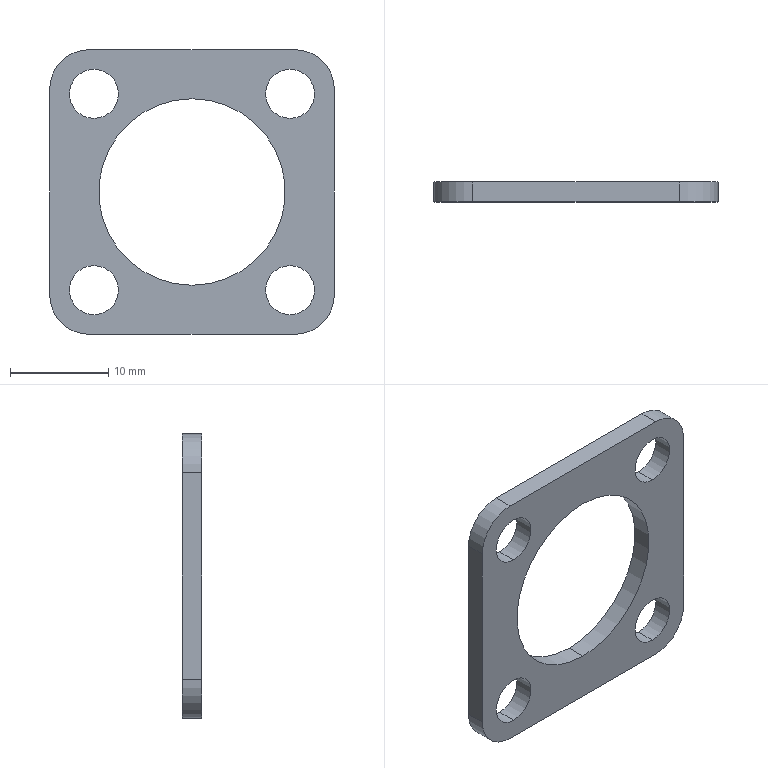Part | NX | features BREP 1 | 1 solid | 20 faces | box 29 x 2 x 29 mm | volume 930.394 mm3 | cylinder 14 | plane 6 | commonest cylinder face diameters 5 x8 8 x4 19 x2
STEP:
#1=CARTESIAN_POINT('',(10.,2.,7.5));
#2=VERTEX_POINT('',#1);
#3=CARTESIAN_POINT('',(10.,2.,12.5));
#4=VERTEX_POINT('',#3);
#5=CARTESIAN_POINT('',(10.,2.,10.));
#6=DIRECTION('',(0.,1.,0.));
#7=DIRECTION('',(1.,0.,0.));
#8=AXIS2_PLACEMENT_3D('',#5,#6,#7);
#9=CIRCLE('',#8,2.5);
#10=EDGE_CURVE('',#2,#4,#9,.T.);
#11=ORIENTED_EDGE('',*,*,#10,.T.);
#12=CARTESIAN_POINT('',(10.,0.,12.5));
#13=VERTEX_POINT('',#12);
#14=CARTESIAN_POINT('',(10.,2.,12.5));
#15=DIRECTION('',(0.,1.,0.));
#16=VECTOR('',#15,1000.);
#17=LINE('',#14,#16);
#18=EDGE_CURVE('',#13,#4,#17,.T.);
#19=ORIENTED_EDGE('',*,*,#18,.F.);
#20=CARTESIAN_POINT('',(10.,0.,7.5));
#21=VERTEX_POINT('',#20);
#22=CARTESIAN_POINT('',(10.,0.,10.));
#23=DIRECTION('',(0.,1.,0.));
#24=DIRECTION('',(1.,0.,0.));
#25=AXIS2_PLACEMENT_3D('',#22,#23,#24);
#26=CIRCLE('',#25,2.5);
#27=EDGE_CURVE('',#21,#13,#26,.T.);
#28=ORIENTED_EDGE('',*,*,#27,.F.);
#29=CARTESIAN_POINT('',(10.,2.,7.5));
#30=DIRECTION('',(0.,1.,0.));
#31=VECTOR('',#30,1000.);
#32=LINE('',#29,#31);
#33=EDGE_CURVE('',#21,#2,#32,.T.);
#34=ORIENTED_EDGE('',*,*,#33,.T.);
#35=EDGE_LOOP('',(#11,#19,#28,#34));
#36=FACE_BOUND('',#35,.T.);
#37=CARTESIAN_POINT('',(10.,2.,10.));
#38=DIRECTION('',(0.,-1.,0.));
#39=DIRECTION('',(0.,0.,-1.));
#40=AXIS2_PLACEMENT_3D('',#37,#38,#39);
#41=CYLINDRICAL_SURFACE('',#40,2.5);
#42=ADVANCED_FACE('',(#36),#41,.F.);
#43=CARTESIAN_POINT('',(10.5,2.,14.5));
#44=VERTEX_POINT('',#43);
#45=CARTESIAN_POINT('',(14.5,2.,10.5));
#46=VERTEX_POINT('',#45);
#47=CARTESIAN_POINT('',(10.5,2.,10.5));
#48=DIRECTION('',(0.,1.,0.));
#49=DIRECTION('',(1.,0.,0.));
#50=AXIS2_PLACEMENT_3D('',#47,#48,#49);
#51=CIRCLE('',#50,4.);
#52=EDGE_CURVE('',#44,#46,#51,.T.);
#53=ORIENTED_EDGE('',*,*,#52,.T.);
#54=CARTESIAN_POINT('',(14.5,2.,-10.5));
#55=VERTEX_POINT('',#54);
#56=CARTESIAN_POINT('',(14.5,2.,0.));
#57=DIRECTION('',(0.,0.,-1.));
#58=VECTOR('',#57,1000.);
#59=LINE('',#56,#58);
#60=EDGE_CURVE('',#46,#55,#59,.T.);
#61=ORIENTED_EDGE('',*,*,#60,.T.);
#62=CARTESIAN_POINT('',(10.5,2.,-14.5));
#63=VERTEX_POINT('',#62);
#64=CARTESIAN_POINT('',(10.5,2.,-10.5));
#65=DIRECTION('',(0.,1.,0.));
#66=DIRECTION('',(1.,0.,0.));
#67=AXIS2_PLACEMENT_3D('',#64,#65,#66);
#68=CIRCLE('',#67,4.);
#69=EDGE_CURVE('',#55,#63,#68,.T.);
#70=ORIENTED_EDGE('',*,*,#69,.T.);
#71=CARTESIAN_POINT('',(-10.5,2.,-14.5));
#72=VERTEX_POINT('',#71);
#73=CARTESIAN_POINT('',(0.,2.,-14.5));
#74=DIRECTION('',(-1.,0.,0.));
#75=VECTOR('',#74,1000.);
#76=LINE('',#73,#75);
#77=EDGE_CURVE('',#63,#72,#76,.T.);
#78=ORIENTED_EDGE('',*,*,#77,.T.);
#79=CARTESIAN_POINT('',(-14.5,2.,-10.5));
#80=VERTEX_POINT('',#79);
#81=CARTESIAN_POINT('',(-10.5,2.,-10.5));
#82=DIRECTION('',(0.,1.,0.));
#83=DIRECTION('',(1.,0.,0.));
#84=AXIS2_PLACEMENT_3D('',#81,#82,#83);
#85=CIRCLE('',#84,4.);
#86=EDGE_CURVE('',#72,#80,#85,.T.);
#87=ORIENTED_EDGE('',*,*,#86,.T.);
#88=CARTESIAN_POINT('',(-14.5,2.,10.5));
#89=VERTEX_POINT('',#88);
#90=CARTESIAN_POINT('',(-14.5,2.,0.));
#91=DIRECTION('',(0.,0.,1.));
#92=VECTOR('',#91,1000.);
#93=LINE('',#90,#92);
#94=EDGE_CURVE('',#80,#89,#93,.T.);
#95=ORIENTED_EDGE('',*,*,#94,.T.);
#96=CARTESIAN_POINT('',(-10.5,2.,14.5));
#97=VERTEX_POINT('',#96);
#98=CARTESIAN_POINT('',(-10.5,2.,10.5));
#99=DIRECTION('',(0.,1.,0.));
#100=DIRECTION('',(1.,0.,0.));
#101=AXIS2_PLACEMENT_3D('',#98,#99,#100);
#102=CIRCLE('',#101,4.);
#103=EDGE_CURVE('',#89,#97,#102,.T.);
#104=ORIENTED_EDGE('',*,*,#103,.T.);
#105=CARTESIAN_POINT('',(0.,2.,14.5));
#106=DIRECTION('',(1.,0.,0.));
#107=VECTOR('',#106,1000.);
#108=LINE('',#105,#107);
#109=EDGE_CURVE('',#97,#44,#108,.T.);
#110=ORIENTED_EDGE('',*,*,#109,.T.);
#111=EDGE_LOOP('',(#53,#61,#70,#78,#87,#95,#104,#110));
#112=FACE_BOUND('',#111,.T.);
#113=CARTESIAN_POINT('',(10.,2.,-12.5));
#114=VERTEX_POINT('',#113);
#115=CARTESIAN_POINT('',(10.,2.,-7.5));
#116=VERTEX_POINT('',#115);
#117=CARTESIAN_POINT('',(10.,2.,-10.));
#118=DIRECTION('',(0.,1.,0.));
#119=DIRECTION('',(1.,0.,0.));
#120=AXIS2_PLACEMENT_3D('',#117,#118,#119);
#121=CIRCLE('',#120,2.5);
#122=EDGE_CURVE('',#114,#116,#121,.T.);
#123=ORIENTED_EDGE('',*,*,#122,.F.);
#124=CARTESIAN_POINT('',(10.,2.,-10.));
#125=DIRECTION('',(0.,1.,0.));
#126=DIRECTION('',(1.,0.,0.));
#127=AXIS2_PLACEMENT_3D('',#124,#125,#126);
#128=CIRCLE('',#127,2.5);
#129=EDGE_CURVE('',#116,#114,#128,.T.);
#130=ORIENTED_EDGE('',*,*,#129,.F.);
#131=EDGE_LOOP('',(#123,#130));
#132=FACE_BOUND('',#131,.T.);
#133=CARTESIAN_POINT('',(-10.,2.,-12.5));
#134=VERTEX_POINT('',#133);
#135=CARTESIAN_POINT('',(-10.,2.,-7.5));
#136=VERTEX_POINT('',#135);
#137=CARTESIAN_POINT('',(-10.,2.,-10.));
#138=DIRECTION('',(0.,1.,0.));
#139=DIRECTION('',(1.,0.,0.));
#140=AXIS2_PLACEMENT_3D('',#137,#138,#139);
#141=CIRCLE('',#140,2.5);
#142=EDGE_CURVE('',#134,#136,#141,.T.);
#143=ORIENTED_EDGE('',*,*,#142,.F.);
#144=CARTESIAN_POINT('',(-10.,2.,-10.));
#145=DIRECTION('',(0.,1.,0.));
#146=DIRECTION('',(1.,0.,0.));
#147=AXIS2_PLACEMENT_3D('',#144,#145,#146);
#148=CIRCLE('',#147,2.5);
#149=EDGE_CURVE('',#136,#134,#148,.T.);
#150=ORIENTED_EDGE('',*,*,#149,.F.);
#151=EDGE_LOOP('',(#143,#150));
#152=FACE_BOUND('',#151,.T.);
#153=CARTESIAN_POINT('',(0.,2.,-9.5));
#154=VERTEX_POINT('',#153);
#155=CARTESIAN_POINT('',(0.,2.,9.5));
#156=VERTEX_POINT('',#155);
#157=CARTESIAN_POINT('',(0.,2.,0.));
#158=DIRECTION('',(0.,1.,0.));
#159=DIRECTION('',(1.,0.,0.));
#160=AXIS2_PLACEMENT_3D('',#157,#158,#159);
#161=CIRCLE('',#160,9.5);
#162=EDGE_CURVE('',#154,#156,#161,.T.);
#163=ORIENTED_EDGE('',*,*,#162,.F.);
#164=CARTESIAN_POINT('',(0.,2.,0.));
#165=DIRECTION('',(0.,1.,0.));
#166=DIRECTION('',(1.,0.,0.));
#167=AXIS2_PLACEMENT_3D('',#164,#165,#166);
#168=CIRCLE('',#167,9.5);
#169=EDGE_CURVE('',#156,#154,#168,.T.);
#170=ORIENTED_EDGE('',*,*,#169,.F.);
#171=EDGE_LOOP('',(#163,#170));
#172=FACE_BOUND('',#171,.T.);
#173=CARTESIAN_POINT('',(-10.,2.,7.5));
#174=VERTEX_POINT('',#173);
#175=CARTESIAN_POINT('',(-10.,2.,12.5));
#176=VERTEX_POINT('',#175);
#177=CARTESIAN_POINT('',(-10.,2.,10.));
#178=DIRECTION('',(0.,1.,0.));
#179=DIRECTION('',(1.,0.,0.));
#180=AXIS2_PLACEMENT_3D('',#177,#178,#179);
#181=CIRCLE('',#180,2.5);
#182=EDGE_CURVE('',#174,#176,#181,.T.);
#183=ORIENTED_EDGE('',*,*,#182,.F.);
#184=CARTESIAN_POINT('',(-10.,2.,10.));
#185=DIRECTION('',(0.,1.,0.));
#186=DIRECTION('',(1.,0.,0.));
#187=AXIS2_PLACEMENT_3D('',#184,#185,#186);
#188=CIRCLE('',#187,2.5);
#189=EDGE_CURVE('',#176,#174,#188,.T.);
#190=ORIENTED_EDGE('',*,*,#189,.F.);
#191=EDGE_LOOP('',(#183,#190));
#192=FACE_BOUND('',#191,.T.);
#193=ORIENTED_EDGE('',*,*,#10,.F.);
#194=CARTESIAN_POINT('',(10.,2.,10.));
#195=DIRECTION('',(0.,1.,0.));
#196=DIRECTION('',(1.,0.,0.));
#197=AXIS2_PLACEMENT_3D('',#194,#195,#196);
#198=CIRCLE('',#197,2.5);
#199=EDGE_CURVE('',#4,#2,#198,.T.);
#200=ORIENTED_EDGE('',*,*,#199,.F.);
#201=EDGE_LOOP('',(#193,#200));
#202=FACE_BOUND('',#201,.T.);
#203=CARTESIAN_POINT('',(10.5,2.,10.5));
#204=DIRECTION('',(0.,1.,0.));
#205=DIRECTION('',(0.,0.,-1.));
#206=AXIS2_PLACEMENT_3D('',#203,#204,#205);
#207=PLANE('',#206);
#208=ADVANCED_FACE('',(#112,#132,#152,#172,#192,#202),#207,.T.);
#209=ORIENTED_EDGE('',*,*,#18,.T.);
#210=ORIENTED_EDGE('',*,*,#199,.T.);
#211=ORIENTED_EDGE('',*,*,#33,.F.);
#212=CARTESIAN_POINT('',(10.,0.,10.));
#213=DIRECTION('',(0.,1.,0.));
#214=DIRECTION('',(1.,0.,0.));
#215=AXIS2_PLACEMENT_3D('',#212,#213,#214);
#216=CIRCLE('',#215,2.5);
#217=EDGE_CURVE('',#13,#21,#216,.T.);
#218=ORIENTED_EDGE('',*,*,#217,.F.);
#219=EDGE_LOOP('',(#209,#210,#211,#218));
#220=FACE_BOUND('',#219,.T.);
#221=CARTESIAN_POINT('',(10.,2.,10.));
#222=DIRECTION('',(0.,-1.,0.));
#223=DIRECTION('',(0.,0.,1.));
#224=AXIS2_PLACEMENT_3D('',#221,#222,#223);
#225=CYLINDRICAL_SURFACE('',#224,2.5);
#226=ADVANCED_FACE('',(#220),#225,.F.);
#227=CARTESIAN_POINT('',(10.5,0.,14.5));
#228=VERTEX_POINT('',#227);
#229=CARTESIAN_POINT('',(14.5,0.,10.5));
#230=VERTEX_POINT('',#229);
#231=CARTESIAN_POINT('',(10.5,0.,10.5));
#232=DIRECTION('',(0.,1.,0.));
#233=DIRECTION('',(1.,0.,0.));
#234=AXIS2_PLACEMENT_3D('',#231,#232,#233);
#235=CIRCLE('',#234,4.);
#236=EDGE_CURVE('',#228,#230,#235,.T.);
#237=ORIENTED_EDGE('',*,*,#236,.F.);
#238=CARTESIAN_POINT('',(-10.5,0.,14.5));
#239=VERTEX_POINT('',#238);
#240=CARTESIAN_POINT('',(0.,0.,14.5));
#241=DIRECTION('',(1.,0.,0.));
#242=VECTOR('',#241,1000.);
#243=LINE('',#240,#242);
#244=EDGE_CURVE('',#239,#228,#243,.T.);
#245=ORIENTED_EDGE('',*,*,#244,.F.);
#246=CARTESIAN_POINT('',(-14.5,0.,10.5));
#247=VERTEX_POINT('',#246);
#248=CARTESIAN_POINT('',(-10.5,0.,10.5));
#249=DIRECTION('',(0.,1.,0.));
#250=DIRECTION('',(1.,0.,0.));
#251=AXIS2_PLACEMENT_3D('',#248,#249,#250);
#252=CIRCLE('',#251,4.);
#253=EDGE_CURVE('',#247,#239,#252,.T.);
#254=ORIENTED_EDGE('',*,*,#253,.F.);
#255=CARTESIAN_POINT('',(-14.5,0.,-10.5));
#256=VERTEX_POINT('',#255);
#257=CARTESIAN_POINT('',(-14.5,0.,0.));
#258=DIRECTION('',(0.,0.,1.));
#259=VECTOR('',#258,1000.);
#260=LINE('',#257,#259);
#261=EDGE_CURVE('',#256,#247,#260,.T.);
#262=ORIENTED_EDGE('',*,*,#261,.F.);
#263=CARTESIAN_POINT('',(-10.5,0.,-14.5));
#264=VERTEX_POINT('',#263);
#265=CARTESIAN_POINT('',(-10.5,0.,-10.5));
#266=DIRECTION('',(0.,1.,0.));
#267=DIRECTION('',(1.,0.,0.));
#268=AXIS2_PLACEMENT_3D('',#265,#266,#267);
#269=CIRCLE('',#268,4.);
#270=EDGE_CURVE('',#264,#256,#269,.T.);
#271=ORIENTED_EDGE('',*,*,#270,.F.);
#272=CARTESIAN_POINT('',(10.5,0.,-14.5));
#273=VERTEX_POINT('',#272);
#274=CARTESIAN_POINT('',(0.,0.,-14.5));
#275=DIRECTION('',(-1.,0.,0.));
#276=VECTOR('',#275,1000.);
#277=LINE('',#274,#276);
#278=EDGE_CURVE('',#273,#264,#277,.T.);
#279=ORIENTED_EDGE('',*,*,#278,.F.);
#280=CARTESIAN_POINT('',(14.5,0.,-10.5));
#281=VERTEX_POINT('',#280);
#282=CARTESIAN_POINT('',(10.5,0.,-10.5));
#283=DIRECTION('',(0.,1.,0.));
#284=DIRECTION('',(1.,0.,0.));
#285=AXIS2_PLACEMENT_3D('',#282,#283,#284);
#286=CIRCLE('',#285,4.);
#287=EDGE_CURVE('',#281,#273,#286,.T.);
#288=ORIENTED_EDGE('',*,*,#287,.F.);
#289=CARTESIAN_POINT('',(14.5,0.,0.));
#290=DIRECTION('',(0.,0.,-1.));
#291=VECTOR('',#290,1000.);
#292=LINE('',#289,#291);
#293=EDGE_CURVE('',#230,#281,#292,.T.);
#294=ORIENTED_EDGE('',*,*,#293,.F.);
#295=EDGE_LOOP('',(#237,#245,#254,#262,#271,#279,#288,#294));
#296=FACE_BOUND('',#295,.T.);
#297=CARTESIAN_POINT('',(0.,0.,-9.5));
#298=VERTEX_POINT('',#297);
#299=CARTESIAN_POINT('',(0.,0.,9.5));
#300=VERTEX_POINT('',#299);
#301=CARTESIAN_POINT('',(0.,0.,0.));
#302=DIRECTION('',(0.,1.,0.));
#303=DIRECTION('',(1.,0.,0.));
#304=AXIS2_PLACEMENT_3D('',#301,#302,#303);
#305=CIRCLE('',#304,9.5);
#306=EDGE_CURVE('',#298,#300,#305,.T.);
#307=ORIENTED_EDGE('',*,*,#306,.T.);
#308=CARTESIAN_POINT('',(0.,0.,0.));
#309=DIRECTION('',(0.,1.,0.));
#310=DIRECTION('',(1.,0.,0.));
#311=AXIS2_PLACEMENT_3D('',#308,#309,#310);
#312=CIRCLE('',#311,9.5);
#313=EDGE_CURVE('',#300,#298,#312,.T.);
#314=ORIENTED_EDGE('',*,*,#313,.T.);
#315=EDGE_LOOP('',(#307,#314));
#316=FACE_BOUND('',#315,.T.);
#317=CARTESIAN_POINT('',(-10.,0.,-12.5));
#318=VERTEX_POINT('',#317);
#319=CARTESIAN_POINT('',(-10.,0.,-7.5));
#320=VERTEX_POINT('',#319);
#321=CARTESIAN_POINT('',(-10.,0.,-10.));
#322=DIRECTION('',(0.,1.,0.));
#323=DIRECTION('',(1.,0.,0.));
#324=AXIS2_PLACEMENT_3D('',#321,#322,#323);
#325=CIRCLE('',#324,2.5);
#326=EDGE_CURVE('',#318,#320,#325,.T.);
#327=ORIENTED_EDGE('',*,*,#326,.T.);
#328=CARTESIAN_POINT('',(-10.,0.,-10.));
#329=DIRECTION('',(0.,1.,0.));
#330=DIRECTION('',(1.,0.,0.));
#331=AXIS2_PLACEMENT_3D('',#328,#329,#330);
#332=CIRCLE('',#331,2.5);
#333=EDGE_CURVE('',#320,#318,#332,.T.);
#334=ORIENTED_EDGE('',*,*,#333,.T.);
#335=EDGE_LOOP('',(#327,#334));
#336=FACE_BOUND('',#335,.T.);
#337=CARTESIAN_POINT('',(-10.,0.,7.5));
#338=VERTEX_POINT('',#337);
#339=CARTESIAN_POINT('',(-10.,0.,12.5));
#340=VERTEX_POINT('',#339);
#341=CARTESIAN_POINT('',(-10.,0.,10.));
#342=DIRECTION('',(0.,1.,0.));
#343=DIRECTION('',(1.,0.,0.));
#344=AXIS2_PLACEMENT_3D('',#341,#342,#343);
#345=CIRCLE('',#344,2.5);
#346=EDGE_CURVE('',#338,#340,#345,.T.);
#347=ORIENTED_EDGE('',*,*,#346,.T.);
#348=CARTESIAN_POINT('',(-10.,0.,10.));
#349=DIRECTION('',(0.,1.,0.));
#350=DIRECTION('',(1.,0.,0.));
#351=AXIS2_PLACEMENT_3D('',#348,#349,#350);
#352=CIRCLE('',#351,2.5);
#353=EDGE_CURVE('',#340,#338,#352,.T.);
#354=ORIENTED_EDGE('',*,*,#353,.T.);
#355=EDGE_LOOP('',(#347,#354));
#356=FACE_BOUND('',#355,.T.);
#357=CARTESIAN_POINT('',(10.,0.,-12.5));
#358=VERTEX_POINT('',#357);
#359=CARTESIAN_POINT('',(10.,0.,-7.5));
#360=VERTEX_POINT('',#359);
#361=CARTESIAN_POINT('',(10.,0.,-10.));
#362=DIRECTION('',(0.,1.,0.));
#363=DIRECTION('',(1.,0.,0.));
#364=AXIS2_PLACEMENT_3D('',#361,#362,#363);
#365=CIRCLE('',#364,2.5);
#366=EDGE_CURVE('',#358,#360,#365,.T.);
#367=ORIENTED_EDGE('',*,*,#366,.T.);
#368=CARTESIAN_POINT('',(10.,0.,-10.));
#369=DIRECTION('',(0.,1.,0.));
#370=DIRECTION('',(1.,0.,0.));
#371=AXIS2_PLACEMENT_3D('',#368,#369,#370);
#372=CIRCLE('',#371,2.5);
#373=EDGE_CURVE('',#360,#358,#372,.T.);
#374=ORIENTED_EDGE('',*,*,#373,.T.);
#375=EDGE_LOOP('',(#367,#374));
#376=FACE_BOUND('',#375,.T.);
#377=ORIENTED_EDGE('',*,*,#27,.T.);
#378=ORIENTED_EDGE('',*,*,#217,.T.);
#379=EDGE_LOOP('',(#377,#378));
#380=FACE_BOUND('',#379,.T.);
#381=CARTESIAN_POINT('',(10.5,0.,10.5));
#382=DIRECTION('',(0.,1.,0.));
#383=DIRECTION('',(0.,0.,-1.));
#384=AXIS2_PLACEMENT_3D('',#381,#382,#383);
#385=PLANE('',#384);
#386=ADVANCED_FACE('',(#296,#316,#336,#356,#376,#380),#385,.F.);
#387=ORIENTED_EDGE('',*,*,#236,.T.);
#388=CARTESIAN_POINT('',(14.5,2.,10.5));
#389=DIRECTION('',(0.,-1.,0.));
#390=VECTOR('',#389,1000.);
#391=LINE('',#388,#390);
#392=EDGE_CURVE('',#46,#230,#391,.T.);
#393=ORIENTED_EDGE('',*,*,#392,.F.);
#394=ORIENTED_EDGE('',*,*,#52,.F.);
#395=CARTESIAN_POINT('',(10.5,2.,14.5));
#396=DIRECTION('',(0.,-1.,0.));
#397=VECTOR('',#396,1000.);
#398=LINE('',#395,#397);
#399=EDGE_CURVE('',#44,#228,#398,.T.);
#400=ORIENTED_EDGE('',*,*,#399,.T.);
#401=EDGE_LOOP('',(#387,#393,#394,#400));
#402=FACE_BOUND('',#401,.T.);
#403=CARTESIAN_POINT('',(10.5,2.,10.5));
#404=DIRECTION('',(0.,-1.,0.));
#405=DIRECTION('',(0.,0.,1.));
#406=AXIS2_PLACEMENT_3D('',#403,#404,#405);
#407=CYLINDRICAL_SURFACE('',#406,4.);
#408=ADVANCED_FACE('',(#402),#407,.T.);
#409=ORIENTED_EDGE('',*,*,#293,.T.);
#410=CARTESIAN_POINT('',(14.5,1.,-10.5));
#411=DIRECTION('',(0.,-1.,0.));
#412=VECTOR('',#411,1000.);
#413=LINE('',#410,#412);
#414=EDGE_CURVE('',#55,#281,#413,.T.);
#415=ORIENTED_EDGE('',*,*,#414,.F.);
#416=ORIENTED_EDGE('',*,*,#60,.F.);
#417=ORIENTED_EDGE('',*,*,#392,.T.);
#418=EDGE_LOOP('',(#409,#415,#416,#417));
#419=FACE_BOUND('',#418,.T.);
#420=CARTESIAN_POINT('',(14.5,2.,10.5));
#421=DIRECTION('',(-1.,0.,0.));
#422=DIRECTION('',(0.,0.,-1.));
#423=AXIS2_PLACEMENT_3D('',#420,#421,#422);
#424=PLANE('',#423);
#425=ADVANCED_FACE('',(#419),#424,.F.);
#426=ORIENTED_EDGE('',*,*,#287,.T.);
#427=CARTESIAN_POINT('',(10.5,2.,-14.5));
#428=DIRECTION('',(0.,-1.,0.));
#429=VECTOR('',#428,1000.);
#430=LINE('',#427,#429);
#431=EDGE_CURVE('',#63,#273,#430,.T.);
#432=ORIENTED_EDGE('',*,*,#431,.F.);
#433=ORIENTED_EDGE('',*,*,#69,.F.);
#434=ORIENTED_EDGE('',*,*,#414,.T.);
#435=EDGE_LOOP('',(#426,#432,#433,#434));
#436=FACE_BOUND('',#435,.T.);
#437=CARTESIAN_POINT('',(10.5,2.,-10.5));
#438=DIRECTION('',(0.,-1.,0.));
#439=DIRECTION('',(0.,0.,1.));
#440=AXIS2_PLACEMENT_3D('',#437,#438,#439);
#441=CYLINDRICAL_SURFACE('',#440,4.);
#442=ADVANCED_FACE('',(#436),#441,.T.);
#443=ORIENTED_EDGE('',*,*,#278,.T.);
#444=CARTESIAN_POINT('',(-10.5,1.,-14.5));
#445=DIRECTION('',(0.,-1.,0.));
#446=VECTOR('',#445,1000.);
#447=LINE('',#444,#446);
#448=EDGE_CURVE('',#72,#264,#447,.T.);
#449=ORIENTED_EDGE('',*,*,#448,.F.);
#450=ORIENTED_EDGE('',*,*,#77,.F.);
#451=ORIENTED_EDGE('',*,*,#431,.T.);
#452=EDGE_LOOP('',(#443,#449,#450,#451));
#453=FACE_BOUND('',#452,.T.);
#454=CARTESIAN_POINT('',(-10.5,2.,-14.5));
#455=DIRECTION('',(0.,0.,1.));
#456=DIRECTION('',(-1.,0.,0.));
#457=AXIS2_PLACEMENT_3D('',#454,#455,#456);
#458=PLANE('',#457);
#459=ADVANCED_FACE('',(#453),#458,.F.);
#460=ORIENTED_EDGE('',*,*,#270,.T.);
#461=CARTESIAN_POINT('',(-14.5,2.,-10.5));
#462=DIRECTION('',(0.,-1.,0.));
#463=VECTOR('',#462,1000.);
#464=LINE('',#461,#463);
#465=EDGE_CURVE('',#80,#256,#464,.T.);
#466=ORIENTED_EDGE('',*,*,#465,.F.);
#467=ORIENTED_EDGE('',*,*,#86,.F.);
#468=ORIENTED_EDGE('',*,*,#448,.T.);
#469=EDGE_LOOP('',(#460,#466,#467,#468));
#470=FACE_BOUND('',#469,.T.);
#471=CARTESIAN_POINT('',(-10.5,2.,-10.5));
#472=DIRECTION('',(0.,-1.,0.));
#473=DIRECTION('',(0.,0.,-1.));
#474=AXIS2_PLACEMENT_3D('',#471,#472,#473);
#475=CYLINDRICAL_SURFACE('',#474,4.);
#476=ADVANCED_FACE('',(#470),#475,.T.);
#477=ORIENTED_EDGE('',*,*,#261,.T.);
#478=CARTESIAN_POINT('',(-14.5,1.,10.5));
#479=DIRECTION('',(0.,-1.,0.));
#480=VECTOR('',#479,1000.);
#481=LINE('',#478,#480);
#482=EDGE_CURVE('',#89,#247,#481,.T.);
#483=ORIENTED_EDGE('',*,*,#482,.F.);
#484=ORIENTED_EDGE('',*,*,#94,.F.);
#485=ORIENTED_EDGE('',*,*,#465,.T.);
#486=EDGE_LOOP('',(#477,#483,#484,#485));
#487=FACE_BOUND('',#486,.T.);
#488=CARTESIAN_POINT('',(-14.5,2.,10.5));
#489=DIRECTION('',(1.,0.,0.));
#490=DIRECTION('',(0.,0.,1.));
#491=AXIS2_PLACEMENT_3D('',#488,#489,#490);
#492=PLANE('',#491);
#493=ADVANCED_FACE('',(#487),#492,.F.);
#494=ORIENTED_EDGE('',*,*,#253,.T.);
#495=CARTESIAN_POINT('',(-10.5,2.,14.5));
#496=DIRECTION('',(0.,-1.,0.));
#497=VECTOR('',#496,1000.);
#498=LINE('',#495,#497);
#499=EDGE_CURVE('',#97,#239,#498,.T.);
#500=ORIENTED_EDGE('',*,*,#499,.F.);
#501=ORIENTED_EDGE('',*,*,#103,.F.);
#502=ORIENTED_EDGE('',*,*,#482,.T.);
#503=EDGE_LOOP('',(#494,#500,#501,#502));
#504=FACE_BOUND('',#503,.T.);
#505=CARTESIAN_POINT('',(-10.5,2.,10.5));
#506=DIRECTION('',(0.,-1.,0.));
#507=DIRECTION('',(0.,0.,-1.));
#508=AXIS2_PLACEMENT_3D('',#505,#506,#507);
#509=CYLINDRICAL_SURFACE('',#508,4.);
#510=ADVANCED_FACE('',(#504),#509,.T.);
#511=ORIENTED_EDGE('',*,*,#244,.T.);
#512=ORIENTED_EDGE('',*,*,#399,.F.);
#513=ORIENTED_EDGE('',*,*,#109,.F.);
#514=ORIENTED_EDGE('',*,*,#499,.T.);
#515=EDGE_LOOP('',(#511,#512,#513,#514));
#516=FACE_BOUND('',#515,.T.);
#517=CARTESIAN_POINT('',(-10.5,2.,14.5));
#518=DIRECTION('',(0.,0.,-1.));
#519=DIRECTION('',(1.,0.,0.));
#520=AXIS2_PLACEMENT_3D('',#517,#518,#519);
#521=PLANE('',#520);
#522=ADVANCED_FACE('',(#516),#521,.F.);
#523=ORIENTED_EDGE('',*,*,#122,.T.);
#524=CARTESIAN_POINT('',(10.,2.,-7.5));
#525=DIRECTION('',(0.,1.,0.));
#526=VECTOR('',#525,1000.);
#527=LINE('',#524,#526);
#528=EDGE_CURVE('',#360,#116,#527,.T.);
#529=ORIENTED_EDGE('',*,*,#528,.F.);
#530=ORIENTED_EDGE('',*,*,#366,.F.);
#531=CARTESIAN_POINT('',(10.,2.,-12.5));
#532=DIRECTION('',(0.,1.,0.));
#533=VECTOR('',#532,1000.);
#534=LINE('',#531,#533);
#535=EDGE_CURVE('',#358,#114,#534,.T.);
#536=ORIENTED_EDGE('',*,*,#535,.T.);
#537=EDGE_LOOP('',(#523,#529,#530,#536));
#538=FACE_BOUND('',#537,.T.);
#539=CARTESIAN_POINT('',(10.,2.,-10.));
#540=DIRECTION('',(0.,-1.,0.));
#541=DIRECTION('',(0.,0.,-1.));
#542=AXIS2_PLACEMENT_3D('',#539,#540,#541);
#543=CYLINDRICAL_SURFACE('',#542,2.5);
#544=ADVANCED_FACE('',(#538),#543,.F.);
#545=ORIENTED_EDGE('',*,*,#528,.T.);
#546=ORIENTED_EDGE('',*,*,#129,.T.);
#547=ORIENTED_EDGE('',*,*,#535,.F.);
#548=ORIENTED_EDGE('',*,*,#373,.F.);
#549=EDGE_LOOP('',(#545,#546,#547,#548));
#550=FACE_BOUND('',#549,.T.);
#551=CARTESIAN_POINT('',(10.,2.,-10.));
#552=DIRECTION('',(0.,-1.,0.));
#553=DIRECTION('',(0.,0.,1.));
#554=AXIS2_PLACEMENT_3D('',#551,#552,#553);
#555=CYLINDRICAL_SURFACE('',#554,2.5);
#556=ADVANCED_FACE('',(#550),#555,.F.);
#557=ORIENTED_EDGE('',*,*,#142,.T.);
#558=CARTESIAN_POINT('',(-10.,2.,-7.5));
#559=DIRECTION('',(0.,1.,0.));
#560=VECTOR('',#559,1000.);
#561=LINE('',#558,#560);
#562=EDGE_CURVE('',#320,#136,#561,.T.);
#563=ORIENTED_EDGE('',*,*,#562,.F.);
#564=ORIENTED_EDGE('',*,*,#326,.F.);
#565=CARTESIAN_POINT('',(-10.,2.,-12.5));
#566=DIRECTION('',(0.,1.,0.));
#567=VECTOR('',#566,1000.);
#568=LINE('',#565,#567);
#569=EDGE_CURVE('',#318,#134,#568,.T.);
#570=ORIENTED_EDGE('',*,*,#569,.T.);
#571=EDGE_LOOP('',(#557,#563,#564,#570));
#572=FACE_BOUND('',#571,.T.);
#573=CARTESIAN_POINT('',(-10.,2.,-10.));
#574=DIRECTION('',(0.,-1.,0.));
#575=DIRECTION('',(0.,0.,-1.));
#576=AXIS2_PLACEMENT_3D('',#573,#574,#575);
#577=CYLINDRICAL_SURFACE('',#576,2.5);
#578=ADVANCED_FACE('',(#572),#577,.F.);
#579=ORIENTED_EDGE('',*,*,#562,.T.);
#580=ORIENTED_EDGE('',*,*,#149,.T.);
#581=ORIENTED_EDGE('',*,*,#569,.F.);
#582=ORIENTED_EDGE('',*,*,#333,.F.);
#583=EDGE_LOOP('',(#579,#580,#581,#582));
#584=FACE_BOUND('',#583,.T.);
#585=CARTESIAN_POINT('',(-10.,2.,-10.));
#586=DIRECTION('',(0.,-1.,0.));
#587=DIRECTION('',(0.,0.,1.));
#588=AXIS2_PLACEMENT_3D('',#585,#586,#587);
#589=CYLINDRICAL_SURFACE('',#588,2.5);
#590=ADVANCED_FACE('',(#584),#589,.F.);
#591=ORIENTED_EDGE('',*,*,#162,.T.);
#592=CARTESIAN_POINT('',(0.,2.,9.5));
#593=DIRECTION('',(0.,1.,0.));
#594=VECTOR('',#593,1000.);
#595=LINE('',#592,#594);
#596=EDGE_CURVE('',#300,#156,#595,.T.);
#597=ORIENTED_EDGE('',*,*,#596,.F.);
#598=ORIENTED_EDGE('',*,*,#306,.F.);
#599=CARTESIAN_POINT('',(0.,2.,-9.5));
#600=DIRECTION('',(0.,1.,0.));
#601=VECTOR('',#600,1000.);
#602=LINE('',#599,#601);
#603=EDGE_CURVE('',#298,#154,#602,.T.);
#604=ORIENTED_EDGE('',*,*,#603,.T.);
#605=EDGE_LOOP('',(#591,#597,#598,#604));
#606=FACE_BOUND('',#605,.T.);
#607=CARTESIAN_POINT('',(0.,2.,0.));
#608=DIRECTION('',(0.,-1.,0.));
#609=DIRECTION('',(0.,0.,-1.));
#610=AXIS2_PLACEMENT_3D('',#607,#608,#609);
#611=CYLINDRICAL_SURFACE('',#610,9.5);
#612=ADVANCED_FACE('',(#606),#611,.F.);
#613=ORIENTED_EDGE('',*,*,#596,.T.);
#614=ORIENTED_EDGE('',*,*,#169,.T.);
#615=ORIENTED_EDGE('',*,*,#603,.F.);
#616=ORIENTED_EDGE('',*,*,#313,.F.);
#617=EDGE_LOOP('',(#613,#614,#615,#616));
#618=FACE_BOUND('',#617,.T.);
#619=CARTESIAN_POINT('',(0.,2.,0.));
#620=DIRECTION('',(0.,-1.,0.));
#621=DIRECTION('',(0.,0.,1.));
#622=AXIS2_PLACEMENT_3D('',#619,#620,#621);
#623=CYLINDRICAL_SURFACE('',#622,9.5);
#624=ADVANCED_FACE('',(#618),#623,.F.);
#625=ORIENTED_EDGE('',*,*,#182,.T.);
#626=CARTESIAN_POINT('',(-10.,2.,12.5));
#627=DIRECTION('',(0.,1.,0.));
#628=VECTOR('',#627,1000.);
#629=LINE('',#626,#628);
#630=EDGE_CURVE('',#340,#176,#629,.T.);
#631=ORIENTED_EDGE('',*,*,#630,.F.);
#632=ORIENTED_EDGE('',*,*,#346,.F.);
#633=CARTESIAN_POINT('',(-10.,2.,7.5));
#634=DIRECTION('',(0.,1.,0.));
#635=VECTOR('',#634,1000.);
#636=LINE('',#633,#635);
#637=EDGE_CURVE('',#338,#174,#636,.T.);
#638=ORIENTED_EDGE('',*,*,#637,.T.);
#639=EDGE_LOOP('',(#625,#631,#632,#638));
#640=FACE_BOUND('',#639,.T.);
#641=CARTESIAN_POINT('',(-10.,2.,10.));
#642=DIRECTION('',(0.,-1.,0.));
#643=DIRECTION('',(0.,0.,-1.));
#644=AXIS2_PLACEMENT_3D('',#641,#642,#643);
#645=CYLINDRICAL_SURFACE('',#644,2.5);
#646=ADVANCED_FACE('',(#640),#645,.F.);
#647=ORIENTED_EDGE('',*,*,#630,.T.);
#648=ORIENTED_EDGE('',*,*,#189,.T.);
#649=ORIENTED_EDGE('',*,*,#637,.F.);
#650=ORIENTED_EDGE('',*,*,#353,.F.);
#651=EDGE_LOOP('',(#647,#648,#649,#650));
#652=FACE_BOUND('',#651,.T.);
#653=CARTESIAN_POINT('',(-10.,2.,10.));
#654=DIRECTION('',(0.,-1.,0.));
#655=DIRECTION('',(0.,0.,1.));
#656=AXIS2_PLACEMENT_3D('',#653,#654,#655);
#657=CYLINDRICAL_SURFACE('',#656,2.5);
#658=ADVANCED_FACE('',(#652),#657,.F.);
#659=CLOSED_SHELL('',(#42,#208,#226,#386,#408,#425,#442,#459,#476,#493,#510,#522,#544,#556,#578,#590,#612,#624,#646,#658));
#660=MANIFOLD_SOLID_BREP('',#659);
#661=(LENGTH_UNIT()NAMED_UNIT(*)SI_UNIT(.MILLI.,.METRE.));
#662=UNCERTAINTY_MEASURE_WITH_UNIT(LENGTH_MEASURE(0.00001),#661,'','');
#663=(NAMED_UNIT(*)PLANE_ANGLE_UNIT()SI_UNIT($,.RADIAN.));
#664=(NAMED_UNIT(*)SI_UNIT($,.STERADIAN.)SOLID_ANGLE_UNIT());
#665=(GEOMETRIC_REPRESENTATION_CONTEXT(3)GLOBAL_UNCERTAINTY_ASSIGNED_CONTEXT((#662))GLOBAL_UNIT_ASSIGNED_CONTEXT((#661,#663,#664))REPRESENTATION_CONTEXT('',''));
#666=ADVANCED_BREP_SHAPE_REPRESENTATION('',(#660),#665);